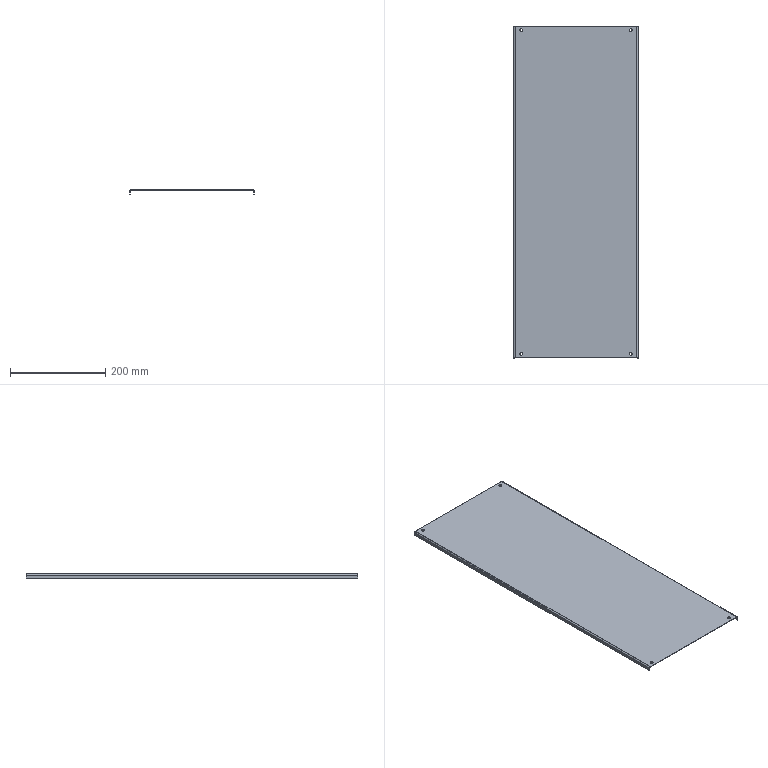Part | STEP file | Vertical arm guard plate (default) | 1 solid | 30 faces | box 262 x 698 x 9 mm | volume 192433 mm3 | plane 18 | cylinder 12 | commonest cylinder face diameters 6 x10 4 x2
STEP:
#1=CARTESIAN_POINT('',(-112.,340.,-1.));
#2=VERTEX_POINT('',#1);
#3=CARTESIAN_POINT('',(-118.,340.,-1.));
#4=VERTEX_POINT('',#3);
#5=CARTESIAN_POINT('',(-115.,340.,-1.));
#6=DIRECTION('',(0.,0.,-1.));
#7=DIRECTION('',(-1.,0.,0.));
#8=AXIS2_PLACEMENT_3D('',#5,#6,#7);
#9=CIRCLE('',#8,3.);
#10=EDGE_CURVE('',#2,#4,#9,.T.);
#11=ORIENTED_EDGE('',*,*,#10,.T.);
#12=CARTESIAN_POINT('',(-118.,340.,0.));
#13=VERTEX_POINT('',#12);
#14=CARTESIAN_POINT('',(-118.,340.,0.));
#15=DIRECTION('',(0.,0.,1.));
#16=VECTOR('',#15,1000.);
#17=LINE('',#14,#16);
#18=EDGE_CURVE('',#4,#13,#17,.T.);
#19=ORIENTED_EDGE('',*,*,#18,.T.);
#20=CARTESIAN_POINT('',(-112.,340.,0.));
#21=VERTEX_POINT('',#20);
#22=CARTESIAN_POINT('',(-115.,340.,0.));
#23=DIRECTION('',(0.,0.,1.));
#24=DIRECTION('',(1.,0.,0.));
#25=AXIS2_PLACEMENT_3D('',#22,#23,#24);
#26=CIRCLE('',#25,3.);
#27=EDGE_CURVE('',#13,#21,#26,.T.);
#28=ORIENTED_EDGE('',*,*,#27,.T.);
#29=CARTESIAN_POINT('',(-112.,340.,0.));
#30=DIRECTION('',(0.,0.,1.));
#31=VECTOR('',#30,1000.);
#32=LINE('',#29,#31);
#33=EDGE_CURVE('',#2,#21,#32,.T.);
#34=ORIENTED_EDGE('',*,*,#33,.F.);
#35=EDGE_LOOP('',(#11,#19,#28,#34));
#36=FACE_OUTER_BOUND('',#35,.T.);
#37=CARTESIAN_POINT('',(-115.,340.,0.));
#38=DIRECTION('',(0.,0.,1.));
#39=DIRECTION('',(1.,0.,0.));
#40=AXIS2_PLACEMENT_3D('',#37,#38,#39);
#41=CYLINDRICAL_SURFACE('',#40,3.);
#42=ADVANCED_FACE('',(#36),#41,.F.);
#43=CARTESIAN_POINT('',(118.,340.,-1.));
#44=VERTEX_POINT('',#43);
#45=CARTESIAN_POINT('',(112.,340.,-1.));
#46=VERTEX_POINT('',#45);
#47=CARTESIAN_POINT('',(115.,340.,-1.));
#48=DIRECTION('',(0.,0.,-1.));
#49=DIRECTION('',(-1.,0.,0.));
#50=AXIS2_PLACEMENT_3D('',#47,#48,#49);
#51=CIRCLE('',#50,3.);
#52=EDGE_CURVE('',#44,#46,#51,.T.);
#53=ORIENTED_EDGE('',*,*,#52,.T.);
#54=CARTESIAN_POINT('',(112.,340.,0.));
#55=VERTEX_POINT('',#54);
#56=CARTESIAN_POINT('',(112.,340.,0.));
#57=DIRECTION('',(0.,0.,1.));
#58=VECTOR('',#57,1000.);
#59=LINE('',#56,#58);
#60=EDGE_CURVE('',#46,#55,#59,.T.);
#61=ORIENTED_EDGE('',*,*,#60,.T.);
#62=CARTESIAN_POINT('',(118.,340.,0.));
#63=VERTEX_POINT('',#62);
#64=CARTESIAN_POINT('',(115.,340.,0.));
#65=DIRECTION('',(0.,0.,1.));
#66=DIRECTION('',(1.,0.,0.));
#67=AXIS2_PLACEMENT_3D('',#64,#65,#66);
#68=CIRCLE('',#67,3.);
#69=EDGE_CURVE('',#55,#63,#68,.T.);
#70=ORIENTED_EDGE('',*,*,#69,.T.);
#71=CARTESIAN_POINT('',(118.,340.,0.));
#72=DIRECTION('',(0.,0.,1.));
#73=VECTOR('',#72,1000.);
#74=LINE('',#71,#73);
#75=EDGE_CURVE('',#44,#63,#74,.T.);
#76=ORIENTED_EDGE('',*,*,#75,.F.);
#77=EDGE_LOOP('',(#53,#61,#70,#76));
#78=FACE_OUTER_BOUND('',#77,.T.);
#79=CARTESIAN_POINT('',(115.,340.,0.));
#80=DIRECTION('',(0.,0.,1.));
#81=DIRECTION('',(1.,0.,0.));
#82=AXIS2_PLACEMENT_3D('',#79,#80,#81);
#83=CYLINDRICAL_SURFACE('',#82,3.);
#84=ADVANCED_FACE('',(#78),#83,.F.);
#85=CARTESIAN_POINT('',(118.,-340.,-1.));
#86=VERTEX_POINT('',#85);
#87=CARTESIAN_POINT('',(112.,-340.,-1.));
#88=VERTEX_POINT('',#87);
#89=CARTESIAN_POINT('',(115.,-340.,-1.));
#90=DIRECTION('',(0.,0.,-1.));
#91=DIRECTION('',(-1.,0.,0.));
#92=AXIS2_PLACEMENT_3D('',#89,#90,#91);
#93=CIRCLE('',#92,3.);
#94=EDGE_CURVE('',#86,#88,#93,.T.);
#95=ORIENTED_EDGE('',*,*,#94,.T.);
#96=CARTESIAN_POINT('',(112.,-340.,0.));
#97=VERTEX_POINT('',#96);
#98=CARTESIAN_POINT('',(112.,-340.,0.));
#99=DIRECTION('',(0.,0.,1.));
#100=VECTOR('',#99,1000.);
#101=LINE('',#98,#100);
#102=EDGE_CURVE('',#88,#97,#101,.T.);
#103=ORIENTED_EDGE('',*,*,#102,.T.);
#104=CARTESIAN_POINT('',(118.,-340.,0.));
#105=VERTEX_POINT('',#104);
#106=CARTESIAN_POINT('',(115.,-340.,0.));
#107=DIRECTION('',(0.,0.,1.));
#108=DIRECTION('',(1.,0.,0.));
#109=AXIS2_PLACEMENT_3D('',#106,#107,#108);
#110=CIRCLE('',#109,3.);
#111=EDGE_CURVE('',#97,#105,#110,.T.);
#112=ORIENTED_EDGE('',*,*,#111,.T.);
#113=CARTESIAN_POINT('',(118.,-340.,0.));
#114=DIRECTION('',(0.,0.,1.));
#115=VECTOR('',#114,1000.);
#116=LINE('',#113,#115);
#117=EDGE_CURVE('',#86,#105,#116,.T.);
#118=ORIENTED_EDGE('',*,*,#117,.F.);
#119=EDGE_LOOP('',(#95,#103,#112,#118));
#120=FACE_OUTER_BOUND('',#119,.T.);
#121=CARTESIAN_POINT('',(115.,-340.,0.));
#122=DIRECTION('',(0.,0.,1.));
#123=DIRECTION('',(1.,0.,0.));
#124=AXIS2_PLACEMENT_3D('',#121,#122,#123);
#125=CYLINDRICAL_SURFACE('',#124,3.);
#126=ADVANCED_FACE('',(#120),#125,.F.);
#127=CARTESIAN_POINT('',(-112.,-340.,-1.));
#128=VERTEX_POINT('',#127);
#129=CARTESIAN_POINT('',(-118.,-340.,-1.));
#130=VERTEX_POINT('',#129);
#131=CARTESIAN_POINT('',(-115.,-340.,-1.));
#132=DIRECTION('',(0.,0.,-1.));
#133=DIRECTION('',(-1.,0.,0.));
#134=AXIS2_PLACEMENT_3D('',#131,#132,#133);
#135=CIRCLE('',#134,3.);
#136=EDGE_CURVE('',#128,#130,#135,.T.);
#137=ORIENTED_EDGE('',*,*,#136,.T.);
#138=CARTESIAN_POINT('',(-118.,-340.,0.));
#139=VERTEX_POINT('',#138);
#140=CARTESIAN_POINT('',(-118.,-340.,0.));
#141=DIRECTION('',(0.,0.,1.));
#142=VECTOR('',#141,1000.);
#143=LINE('',#140,#142);
#144=EDGE_CURVE('',#130,#139,#143,.T.);
#145=ORIENTED_EDGE('',*,*,#144,.T.);
#146=CARTESIAN_POINT('',(-112.,-340.,0.));
#147=VERTEX_POINT('',#146);
#148=CARTESIAN_POINT('',(-115.,-340.,0.));
#149=DIRECTION('',(0.,0.,1.));
#150=DIRECTION('',(1.,0.,0.));
#151=AXIS2_PLACEMENT_3D('',#148,#149,#150);
#152=CIRCLE('',#151,3.);
#153=EDGE_CURVE('',#139,#147,#152,.T.);
#154=ORIENTED_EDGE('',*,*,#153,.T.);
#155=CARTESIAN_POINT('',(-112.,-340.,0.));
#156=DIRECTION('',(0.,0.,1.));
#157=VECTOR('',#156,1000.);
#158=LINE('',#155,#157);
#159=EDGE_CURVE('',#128,#147,#158,.T.);
#160=ORIENTED_EDGE('',*,*,#159,.F.);
#161=EDGE_LOOP('',(#137,#145,#154,#160));
#162=FACE_OUTER_BOUND('',#161,.T.);
#163=CARTESIAN_POINT('',(-115.,-340.,0.));
#164=DIRECTION('',(0.,0.,1.));
#165=DIRECTION('',(1.,0.,0.));
#166=AXIS2_PLACEMENT_3D('',#163,#164,#165);
#167=CYLINDRICAL_SURFACE('',#166,3.);
#168=ADVANCED_FACE('',(#162),#167,.F.);
#169=ORIENTED_EDGE('',*,*,#10,.F.);
#170=CARTESIAN_POINT('',(-115.,340.,-1.));
#171=DIRECTION('',(0.,0.,-1.));
#172=DIRECTION('',(-1.,0.,0.));
#173=AXIS2_PLACEMENT_3D('',#170,#171,#172);
#174=CIRCLE('',#173,3.);
#175=EDGE_CURVE('',#4,#2,#174,.T.);
#176=ORIENTED_EDGE('',*,*,#175,.F.);
#177=EDGE_LOOP('',(#169,#176));
#178=FACE_BOUND('',#177,.T.);
#179=ORIENTED_EDGE('',*,*,#52,.F.);
#180=CARTESIAN_POINT('',(115.,340.,-1.));
#181=DIRECTION('',(0.,0.,-1.));
#182=DIRECTION('',(-1.,0.,0.));
#183=AXIS2_PLACEMENT_3D('',#180,#181,#182);
#184=CIRCLE('',#183,3.);
#185=EDGE_CURVE('',#46,#44,#184,.T.);
#186=ORIENTED_EDGE('',*,*,#185,.F.);
#187=EDGE_LOOP('',(#179,#186));
#188=FACE_BOUND('',#187,.T.);
#189=ORIENTED_EDGE('',*,*,#94,.F.);
#190=CARTESIAN_POINT('',(115.,-340.,-1.));
#191=DIRECTION('',(0.,0.,-1.));
#192=DIRECTION('',(-1.,0.,0.));
#193=AXIS2_PLACEMENT_3D('',#190,#191,#192);
#194=CIRCLE('',#193,3.);
#195=EDGE_CURVE('',#88,#86,#194,.T.);
#196=ORIENTED_EDGE('',*,*,#195,.F.);
#197=EDGE_LOOP('',(#189,#196));
#198=FACE_BOUND('',#197,.T.);
#199=ORIENTED_EDGE('',*,*,#136,.F.);
#200=CARTESIAN_POINT('',(-115.,-340.,-1.));
#201=DIRECTION('',(0.,0.,-1.));
#202=DIRECTION('',(-1.,0.,0.));
#203=AXIS2_PLACEMENT_3D('',#200,#201,#202);
#204=CIRCLE('',#203,3.);
#205=EDGE_CURVE('',#130,#128,#204,.T.);
#206=ORIENTED_EDGE('',*,*,#205,.F.);
#207=EDGE_LOOP('',(#199,#206));
#208=FACE_BOUND('',#207,.T.);
#209=CARTESIAN_POINT('',(-128.,-349.,-1.));
#210=VERTEX_POINT('',#209);
#211=CARTESIAN_POINT('',(128.,-349.,-1.));
#212=VERTEX_POINT('',#211);
#213=CARTESIAN_POINT('',(-130.,-349.,-1.));
#214=DIRECTION('',(1.,0.,0.));
#215=VECTOR('',#214,1000.);
#216=LINE('',#213,#215);
#217=EDGE_CURVE('',#210,#212,#216,.T.);
#218=ORIENTED_EDGE('',*,*,#217,.F.);
#219=CARTESIAN_POINT('',(-128.,349.,-1.));
#220=VERTEX_POINT('',#219);
#221=CARTESIAN_POINT('',(-128.,349.,-1.));
#222=DIRECTION('',(0.,-1.,0.));
#223=VECTOR('',#222,1000.);
#224=LINE('',#221,#223);
#225=EDGE_CURVE('',#220,#210,#224,.T.);
#226=ORIENTED_EDGE('',*,*,#225,.F.);
#227=CARTESIAN_POINT('',(128.,349.,-1.));
#228=VERTEX_POINT('',#227);
#229=CARTESIAN_POINT('',(-130.,349.,-1.));
#230=DIRECTION('',(-1.,0.,0.));
#231=VECTOR('',#230,1000.);
#232=LINE('',#229,#231);
#233=EDGE_CURVE('',#228,#220,#232,.T.);
#234=ORIENTED_EDGE('',*,*,#233,.F.);
#235=CARTESIAN_POINT('',(128.,-349.,-1.));
#236=DIRECTION('',(0.,1.,0.));
#237=VECTOR('',#236,1000.);
#238=LINE('',#235,#237);
#239=EDGE_CURVE('',#212,#228,#238,.T.);
#240=ORIENTED_EDGE('',*,*,#239,.F.);
#241=EDGE_LOOP('',(#218,#226,#234,#240));
#242=FACE_OUTER_BOUND('',#241,.T.);
#243=CARTESIAN_POINT('',(130.,349.,-1.));
#244=DIRECTION('',(0.,0.,-1.));
#245=DIRECTION('',(-1.,0.,0.));
#246=AXIS2_PLACEMENT_3D('',#243,#244,#245);
#247=PLANE('',#246);
#248=ADVANCED_FACE('',(#178,#188,#198,#208,#242),#247,.T.);
#249=CARTESIAN_POINT('',(-115.,340.,0.));
#250=DIRECTION('',(0.,0.,1.));
#251=DIRECTION('',(1.,0.,0.));
#252=AXIS2_PLACEMENT_3D('',#249,#250,#251);
#253=CIRCLE('',#252,3.);
#254=EDGE_CURVE('',#21,#13,#253,.T.);
#255=ORIENTED_EDGE('',*,*,#254,.F.);
#256=ORIENTED_EDGE('',*,*,#27,.F.);
#257=EDGE_LOOP('',(#255,#256));
#258=FACE_BOUND('',#257,.T.);
#259=CARTESIAN_POINT('',(115.,340.,0.));
#260=DIRECTION('',(0.,0.,1.));
#261=DIRECTION('',(1.,0.,0.));
#262=AXIS2_PLACEMENT_3D('',#259,#260,#261);
#263=CIRCLE('',#262,3.);
#264=EDGE_CURVE('',#63,#55,#263,.T.);
#265=ORIENTED_EDGE('',*,*,#264,.F.);
#266=ORIENTED_EDGE('',*,*,#69,.F.);
#267=EDGE_LOOP('',(#265,#266));
#268=FACE_BOUND('',#267,.T.);
#269=CARTESIAN_POINT('',(115.,-340.,0.));
#270=DIRECTION('',(0.,0.,1.));
#271=DIRECTION('',(1.,0.,0.));
#272=AXIS2_PLACEMENT_3D('',#269,#270,#271);
#273=CIRCLE('',#272,3.);
#274=EDGE_CURVE('',#105,#97,#273,.T.);
#275=ORIENTED_EDGE('',*,*,#274,.F.);
#276=ORIENTED_EDGE('',*,*,#111,.F.);
#277=EDGE_LOOP('',(#275,#276));
#278=FACE_BOUND('',#277,.T.);
#279=CARTESIAN_POINT('',(-115.,-340.,0.));
#280=DIRECTION('',(0.,0.,1.));
#281=DIRECTION('',(1.,0.,0.));
#282=AXIS2_PLACEMENT_3D('',#279,#280,#281);
#283=CIRCLE('',#282,3.);
#284=EDGE_CURVE('',#147,#139,#283,.T.);
#285=ORIENTED_EDGE('',*,*,#284,.F.);
#286=ORIENTED_EDGE('',*,*,#153,.F.);
#287=EDGE_LOOP('',(#285,#286));
#288=FACE_BOUND('',#287,.T.);
#289=CARTESIAN_POINT('',(-128.,349.,0.));
#290=VERTEX_POINT('',#289);
#291=CARTESIAN_POINT('',(-128.,-349.,0.));
#292=VERTEX_POINT('',#291);
#293=CARTESIAN_POINT('',(-128.,349.,0.));
#294=DIRECTION('',(0.,-1.,0.));
#295=VECTOR('',#294,1000.);
#296=LINE('',#293,#295);
#297=EDGE_CURVE('',#290,#292,#296,.T.);
#298=ORIENTED_EDGE('',*,*,#297,.T.);
#299=CARTESIAN_POINT('',(128.,-349.,0.));
#300=VERTEX_POINT('',#299);
#301=CARTESIAN_POINT('',(-130.,-349.,0.));
#302=DIRECTION('',(1.,0.,0.));
#303=VECTOR('',#302,1000.);
#304=LINE('',#301,#303);
#305=EDGE_CURVE('',#292,#300,#304,.T.);
#306=ORIENTED_EDGE('',*,*,#305,.T.);
#307=CARTESIAN_POINT('',(128.,349.,0.));
#308=VERTEX_POINT('',#307);
#309=CARTESIAN_POINT('',(128.,-349.,0.));
#310=DIRECTION('',(0.,1.,0.));
#311=VECTOR('',#310,1000.);
#312=LINE('',#309,#311);
#313=EDGE_CURVE('',#300,#308,#312,.T.);
#314=ORIENTED_EDGE('',*,*,#313,.T.);
#315=CARTESIAN_POINT('',(-130.,349.,0.));
#316=DIRECTION('',(-1.,0.,0.));
#317=VECTOR('',#316,1000.);
#318=LINE('',#315,#317);
#319=EDGE_CURVE('',#308,#290,#318,.T.);
#320=ORIENTED_EDGE('',*,*,#319,.T.);
#321=EDGE_LOOP('',(#298,#306,#314,#320));
#322=FACE_OUTER_BOUND('',#321,.T.);
#323=CARTESIAN_POINT('',(130.,349.,0.));
#324=DIRECTION('',(0.,0.,-1.));
#325=DIRECTION('',(-1.,0.,0.));
#326=AXIS2_PLACEMENT_3D('',#323,#324,#325);
#327=PLANE('',#326);
#328=ADVANCED_FACE('',(#258,#268,#278,#288,#322),#327,.F.);
#329=ORIENTED_EDGE('',*,*,#233,.T.);
#330=CARTESIAN_POINT('',(-128.,349.,-1.));
#331=DIRECTION('',(0.,0.,1.));
#332=VECTOR('',#331,1000.);
#333=LINE('',#330,#332);
#334=EDGE_CURVE('',#220,#290,#333,.T.);
#335=ORIENTED_EDGE('',*,*,#334,.T.);
#336=ORIENTED_EDGE('',*,*,#319,.F.);
#337=CARTESIAN_POINT('',(128.,349.,-1.));
#338=DIRECTION('',(0.,0.,1.));
#339=VECTOR('',#338,1000.);
#340=LINE('',#337,#339);
#341=EDGE_CURVE('',#228,#308,#340,.T.);
#342=ORIENTED_EDGE('',*,*,#341,.F.);
#343=EDGE_LOOP('',(#329,#335,#336,#342));
#344=FACE_OUTER_BOUND('',#343,.T.);
#345=CARTESIAN_POINT('',(-130.,349.,-1.));
#346=DIRECTION('',(0.,1.,0.));
#347=DIRECTION('',(0.,0.,1.));
#348=AXIS2_PLACEMENT_3D('',#345,#346,#347);
#349=PLANE('',#348);
#350=ADVANCED_FACE('',(#344),#349,.T.);
#351=CARTESIAN_POINT('',(-128.,-349.,-1.));
#352=DIRECTION('',(0.,0.,1.));
#353=VECTOR('',#352,1000.);
#354=LINE('',#351,#353);
#355=EDGE_CURVE('',#210,#292,#354,.T.);
#356=ORIENTED_EDGE('',*,*,#355,.F.);
#357=ORIENTED_EDGE('',*,*,#217,.T.);
#358=CARTESIAN_POINT('',(128.,-349.,-1.));
#359=DIRECTION('',(0.,0.,1.));
#360=VECTOR('',#359,1000.);
#361=LINE('',#358,#360);
#362=EDGE_CURVE('',#212,#300,#361,.T.);
#363=ORIENTED_EDGE('',*,*,#362,.T.);
#364=ORIENTED_EDGE('',*,*,#305,.F.);
#365=EDGE_LOOP('',(#356,#357,#363,#364));
#366=FACE_OUTER_BOUND('',#365,.T.);
#367=CARTESIAN_POINT('',(-130.,-349.,-1.));
#368=DIRECTION('',(0.,-1.,0.));
#369=DIRECTION('',(0.,0.,-1.));
#370=AXIS2_PLACEMENT_3D('',#367,#368,#369);
#371=PLANE('',#370);
#372=ADVANCED_FACE('',(#366),#371,.T.);
#373=ORIENTED_EDGE('',*,*,#144,.F.);
#374=ORIENTED_EDGE('',*,*,#205,.T.);
#375=ORIENTED_EDGE('',*,*,#159,.T.);
#376=ORIENTED_EDGE('',*,*,#284,.T.);
#377=EDGE_LOOP('',(#373,#374,#375,#376));
#378=FACE_OUTER_BOUND('',#377,.T.);
#379=CARTESIAN_POINT('',(-115.,-340.,0.));
#380=DIRECTION('',(0.,0.,1.));
#381=DIRECTION('',(1.,0.,0.));
#382=AXIS2_PLACEMENT_3D('',#379,#380,#381);
#383=CYLINDRICAL_SURFACE('',#382,3.);
#384=ADVANCED_FACE('',(#378),#383,.F.);
#385=ORIENTED_EDGE('',*,*,#102,.F.);
#386=ORIENTED_EDGE('',*,*,#195,.T.);
#387=ORIENTED_EDGE('',*,*,#117,.T.);
#388=ORIENTED_EDGE('',*,*,#274,.T.);
#389=EDGE_LOOP('',(#385,#386,#387,#388));
#390=FACE_OUTER_BOUND('',#389,.T.);
#391=CARTESIAN_POINT('',(115.,-340.,0.));
#392=DIRECTION('',(0.,0.,1.));
#393=DIRECTION('',(1.,0.,0.));
#394=AXIS2_PLACEMENT_3D('',#391,#392,#393);
#395=CYLINDRICAL_SURFACE('',#394,3.);
#396=ADVANCED_FACE('',(#390),#395,.F.);
#397=ORIENTED_EDGE('',*,*,#60,.F.);
#398=ORIENTED_EDGE('',*,*,#185,.T.);
#399=ORIENTED_EDGE('',*,*,#75,.T.);
#400=ORIENTED_EDGE('',*,*,#264,.T.);
#401=EDGE_LOOP('',(#397,#398,#399,#400));
#402=FACE_OUTER_BOUND('',#401,.T.);
#403=CARTESIAN_POINT('',(115.,340.,0.));
#404=DIRECTION('',(0.,0.,1.));
#405=DIRECTION('',(1.,0.,0.));
#406=AXIS2_PLACEMENT_3D('',#403,#404,#405);
#407=CYLINDRICAL_SURFACE('',#406,3.);
#408=ADVANCED_FACE('',(#402),#407,.F.);
#409=ORIENTED_EDGE('',*,*,#18,.F.);
#410=ORIENTED_EDGE('',*,*,#175,.T.);
#411=ORIENTED_EDGE('',*,*,#33,.T.);
#412=ORIENTED_EDGE('',*,*,#254,.T.);
#413=EDGE_LOOP('',(#409,#410,#411,#412));
#414=FACE_OUTER_BOUND('',#413,.T.);
#415=CARTESIAN_POINT('',(-115.,340.,0.));
#416=DIRECTION('',(0.,0.,1.));
#417=DIRECTION('',(1.,0.,0.));
#418=AXIS2_PLACEMENT_3D('',#415,#416,#417);
#419=CYLINDRICAL_SURFACE('',#418,3.);
#420=ADVANCED_FACE('',(#414),#419,.F.);
#421=CARTESIAN_POINT('',(130.,349.,-3.));
#422=VERTEX_POINT('',#421);
#423=CARTESIAN_POINT('',(131.,349.,-3.));
#424=VERTEX_POINT('',#423);
#425=CARTESIAN_POINT('',(130.,349.,-3.));
#426=DIRECTION('',(1.,0.,0.));
#427=VECTOR('',#426,1000.);
#428=LINE('',#425,#427);
#429=EDGE_CURVE('',#422,#424,#428,.T.);
#430=ORIENTED_EDGE('',*,*,#429,.F.);
#431=CARTESIAN_POINT('',(128.,349.,-3.));
#432=DIRECTION('',(0.,1.,0.));
#433=DIRECTION('',(0.,0.,-1.));
#434=AXIS2_PLACEMENT_3D('',#431,#432,#433);
#435=CIRCLE('',#434,2.);
#436=EDGE_CURVE('',#228,#422,#435,.T.);
#437=ORIENTED_EDGE('',*,*,#436,.F.);
#438=ORIENTED_EDGE('',*,*,#341,.T.);
#439=CARTESIAN_POINT('',(128.,349.,-3.));
#440=DIRECTION('',(0.,1.,0.));
#441=DIRECTION('',(0.,0.,-1.));
#442=AXIS2_PLACEMENT_3D('',#439,#440,#441);
#443=CIRCLE('',#442,3.);
#444=EDGE_CURVE('',#308,#424,#443,.T.);
#445=ORIENTED_EDGE('',*,*,#444,.T.);
#446=EDGE_LOOP('',(#430,#437,#438,#445));
#447=FACE_OUTER_BOUND('',#446,.T.);
#448=CARTESIAN_POINT('',(128.,349.,-3.));
#449=DIRECTION('',(0.,1.,0.));
#450=DIRECTION('',(0.,0.,1.));
#451=AXIS2_PLACEMENT_3D('',#448,#449,#450);
#452=PLANE('',#451);
#453=ADVANCED_FACE('',(#447),#452,.T.);
#454=CARTESIAN_POINT('',(130.,-349.,-3.));
#455=VERTEX_POINT('',#454);
#456=CARTESIAN_POINT('',(128.,-349.,-3.));
#457=DIRECTION('',(0.,-1.,0.));
#458=DIRECTION('',(0.,0.,-1.));
#459=AXIS2_PLACEMENT_3D('',#456,#457,#458);
#460=CIRCLE('',#459,2.);
#461=EDGE_CURVE('',#455,#212,#460,.T.);
#462=ORIENTED_EDGE('',*,*,#461,.F.);
#463=CARTESIAN_POINT('',(131.,-349.,-3.));
#464=VERTEX_POINT('',#463);
#465=CARTESIAN_POINT('',(130.,-349.,-3.));
#466=DIRECTION('',(1.,0.,0.));
#467=VECTOR('',#466,1000.);
#468=LINE('',#465,#467);
#469=EDGE_CURVE('',#455,#464,#468,.T.);
#470=ORIENTED_EDGE('',*,*,#469,.T.);
#471=CARTESIAN_POINT('',(128.,-349.,-3.));
#472=DIRECTION('',(0.,-1.,0.));
#473=DIRECTION('',(0.,0.,-1.));
#474=AXIS2_PLACEMENT_3D('',#471,#472,#473);
#475=CIRCLE('',#474,3.);
#476=EDGE_CURVE('',#464,#300,#475,.T.);
#477=ORIENTED_EDGE('',*,*,#476,.T.);
#478=ORIENTED_EDGE('',*,*,#362,.F.);
#479=EDGE_LOOP('',(#462,#470,#477,#478));
#480=FACE_OUTER_BOUND('',#479,.T.);
#481=CARTESIAN_POINT('',(128.,-349.,-3.));
#482=DIRECTION('',(0.,1.,0.));
#483=DIRECTION('',(0.,0.,1.));
#484=AXIS2_PLACEMENT_3D('',#481,#482,#483);
#485=PLANE('',#484);
#486=ADVANCED_FACE('',(#480),#485,.F.);
#487=ORIENTED_EDGE('',*,*,#313,.F.);
#488=ORIENTED_EDGE('',*,*,#476,.F.);
#489=CARTESIAN_POINT('',(131.,-349.,-3.));
#490=DIRECTION('',(0.,-1.,0.));
#491=VECTOR('',#490,1000.);
#492=LINE('',#489,#491);
#493=EDGE_CURVE('',#424,#464,#492,.T.);
#494=ORIENTED_EDGE('',*,*,#493,.F.);
#495=ORIENTED_EDGE('',*,*,#444,.F.);
#496=EDGE_LOOP('',(#487,#488,#494,#495));
#497=FACE_OUTER_BOUND('',#496,.T.);
#498=CARTESIAN_POINT('',(128.,-349.,-3.));
#499=DIRECTION('',(0.,-1.,0.));
#500=DIRECTION('',(1.,0.,0.));
#501=AXIS2_PLACEMENT_3D('',#498,#499,#500);
#502=CYLINDRICAL_SURFACE('',#501,3.);
#503=ADVANCED_FACE('',(#497),#502,.T.);
#504=ORIENTED_EDGE('',*,*,#239,.T.);
#505=ORIENTED_EDGE('',*,*,#436,.T.);
#506=CARTESIAN_POINT('',(130.,349.,-3.));
#507=DIRECTION('',(0.,-1.,0.));
#508=VECTOR('',#507,1000.);
#509=LINE('',#506,#508);
#510=EDGE_CURVE('',#422,#455,#509,.T.);
#511=ORIENTED_EDGE('',*,*,#510,.T.);
#512=ORIENTED_EDGE('',*,*,#461,.T.);
#513=EDGE_LOOP('',(#504,#505,#511,#512));
#514=FACE_OUTER_BOUND('',#513,.T.);
#515=CARTESIAN_POINT('',(128.,-349.,-3.));
#516=DIRECTION('',(0.,-1.,0.));
#517=DIRECTION('',(1.,0.,0.));
#518=AXIS2_PLACEMENT_3D('',#515,#516,#517);
#519=CYLINDRICAL_SURFACE('',#518,2.);
#520=ADVANCED_FACE('',(#514),#519,.F.);
#521=CARTESIAN_POINT('',(131.,-349.,-9.));
#522=VERTEX_POINT('',#521);
#523=CARTESIAN_POINT('',(131.,-349.,-1.));
#524=DIRECTION('',(0.,0.,1.));
#525=VECTOR('',#524,1000.);
#526=LINE('',#523,#525);
#527=EDGE_CURVE('',#522,#464,#526,.T.);
#528=ORIENTED_EDGE('',*,*,#527,.T.);
#529=ORIENTED_EDGE('',*,*,#469,.F.);
#530=CARTESIAN_POINT('',(130.,-349.,-9.));
#531=VERTEX_POINT('',#530);
#532=CARTESIAN_POINT('',(130.,-349.,-1.));
#533=DIRECTION('',(0.,0.,1.));
#534=VECTOR('',#533,1000.);
#535=LINE('',#532,#534);
#536=EDGE_CURVE('',#531,#455,#535,.T.);
#537=ORIENTED_EDGE('',*,*,#536,.F.);
#538=CARTESIAN_POINT('',(131.,-349.,-9.));
#539=DIRECTION('',(-1.,0.,0.));
#540=VECTOR('',#539,1000.);
#541=LINE('',#538,#540);
#542=EDGE_CURVE('',#522,#531,#541,.T.);
#543=ORIENTED_EDGE('',*,*,#542,.F.);
#544=EDGE_LOOP('',(#528,#529,#537,#543));
#545=FACE_OUTER_BOUND('',#544,.T.);
#546=CARTESIAN_POINT('',(131.,-349.,-1.));
#547=DIRECTION('',(0.,-1.,0.));
#548=DIRECTION('',(0.,0.,-1.));
#549=AXIS2_PLACEMENT_3D('',#546,#547,#548);
#550=PLANE('',#549);
#551=ADVANCED_FACE('',(#545),#550,.T.);
#552=CARTESIAN_POINT('',(130.,349.,-9.));
#553=VERTEX_POINT('',#552);
#554=CARTESIAN_POINT('',(130.,349.,-9.));
#555=DIRECTION('',(0.,0.,-1.));
#556=VECTOR('',#555,1000.);
#557=LINE('',#554,#556);
#558=EDGE_CURVE('',#422,#553,#557,.T.);
#559=ORIENTED_EDGE('',*,*,#558,.F.);
#560=ORIENTED_EDGE('',*,*,#429,.T.);
#561=CARTESIAN_POINT('',(131.,349.,-9.));
#562=VERTEX_POINT('',#561);
#563=CARTESIAN_POINT('',(131.,349.,-9.));
#564=DIRECTION('',(0.,0.,-1.));
#565=VECTOR('',#564,1000.);
#566=LINE('',#563,#565);
#567=EDGE_CURVE('',#424,#562,#566,.T.);
#568=ORIENTED_EDGE('',*,*,#567,.T.);
#569=CARTESIAN_POINT('',(131.,349.,-9.));
#570=DIRECTION('',(-1.,0.,0.));
#571=VECTOR('',#570,1000.);
#572=LINE('',#569,#571);
#573=EDGE_CURVE('',#562,#553,#572,.T.);
#574=ORIENTED_EDGE('',*,*,#573,.T.);
#575=EDGE_LOOP('',(#559,#560,#568,#574));
#576=FACE_OUTER_BOUND('',#575,.T.);
#577=CARTESIAN_POINT('',(131.,349.,-9.));
#578=DIRECTION('',(0.,1.,0.));
#579=DIRECTION('',(0.,0.,1.));
#580=AXIS2_PLACEMENT_3D('',#577,#578,#579);
#581=PLANE('',#580);
#582=ADVANCED_FACE('',(#576),#581,.T.);
#583=ORIENTED_EDGE('',*,*,#567,.F.);
#584=ORIENTED_EDGE('',*,*,#493,.T.);
#585=ORIENTED_EDGE('',*,*,#527,.F.);
#586=CARTESIAN_POINT('',(131.,-349.,-9.));
#587=DIRECTION('',(0.,-1.,0.));
#588=VECTOR('',#587,1000.);
#589=LINE('',#586,#588);
#590=EDGE_CURVE('',#562,#522,#589,.T.);
#591=ORIENTED_EDGE('',*,*,#590,.F.);
#592=EDGE_LOOP('',(#583,#584,#585,#591));
#593=FACE_OUTER_BOUND('',#592,.T.);
#594=CARTESIAN_POINT('',(131.,-349.,-1.));
#595=DIRECTION('',(1.,0.,0.));
#596=DIRECTION('',(0.,0.,-1.));
#597=AXIS2_PLACEMENT_3D('',#594,#595,#596);
#598=PLANE('',#597);
#599=ADVANCED_FACE('',(#593),#598,.T.);
#600=ORIENTED_EDGE('',*,*,#510,.F.);
#601=ORIENTED_EDGE('',*,*,#558,.T.);
#602=CARTESIAN_POINT('',(130.,-349.,-9.));
#603=DIRECTION('',(0.,-1.,0.));
#604=VECTOR('',#603,1000.);
#605=LINE('',#602,#604);
#606=EDGE_CURVE('',#553,#531,#605,.T.);
#607=ORIENTED_EDGE('',*,*,#606,.T.);
#608=ORIENTED_EDGE('',*,*,#536,.T.);
#609=EDGE_LOOP('',(#600,#601,#607,#608));
#610=FACE_OUTER_BOUND('',#609,.T.);
#611=CARTESIAN_POINT('',(130.,-349.,-1.));
#612=DIRECTION('',(1.,0.,0.));
#613=DIRECTION('',(0.,0.,-1.));
#614=AXIS2_PLACEMENT_3D('',#611,#612,#613);
#615=PLANE('',#614);
#616=ADVANCED_FACE('',(#610),#615,.F.);
#617=ORIENTED_EDGE('',*,*,#606,.F.);
#618=ORIENTED_EDGE('',*,*,#573,.F.);
#619=ORIENTED_EDGE('',*,*,#590,.T.);
#620=ORIENTED_EDGE('',*,*,#542,.T.);
#621=EDGE_LOOP('',(#617,#618,#619,#620));
#622=FACE_OUTER_BOUND('',#621,.T.);
#623=CARTESIAN_POINT('',(131.,-349.,-9.));
#624=DIRECTION('',(0.,0.,-1.));
#625=DIRECTION('',(-1.,0.,0.));
#626=AXIS2_PLACEMENT_3D('',#623,#624,#625);
#627=PLANE('',#626);
#628=ADVANCED_FACE('',(#622),#627,.T.);
#629=CARTESIAN_POINT('',(-130.,-349.,-3.));
#630=VERTEX_POINT('',#629);
#631=CARTESIAN_POINT('',(-131.,-349.,-3.));
#632=VERTEX_POINT('',#631);
#633=CARTESIAN_POINT('',(-130.,-349.,-3.));
#634=DIRECTION('',(-1.,0.,0.));
#635=VECTOR('',#634,1000.);
#636=LINE('',#633,#635);
#637=EDGE_CURVE('',#630,#632,#636,.T.);
#638=ORIENTED_EDGE('',*,*,#637,.F.);
#639=CARTESIAN_POINT('',(-128.,-349.,-3.));
#640=DIRECTION('',(0.,-1.,0.));
#641=DIRECTION('',(0.,0.,1.));
#642=AXIS2_PLACEMENT_3D('',#639,#640,#641);
#643=CIRCLE('',#642,2.);
#644=EDGE_CURVE('',#210,#630,#643,.T.);
#645=ORIENTED_EDGE('',*,*,#644,.F.);
#646=ORIENTED_EDGE('',*,*,#355,.T.);
#647=CARTESIAN_POINT('',(-128.,-349.,-3.));
#648=DIRECTION('',(0.,-1.,0.));
#649=DIRECTION('',(0.,0.,1.));
#650=AXIS2_PLACEMENT_3D('',#647,#648,#649);
#651=CIRCLE('',#650,3.);
#652=EDGE_CURVE('',#292,#632,#651,.T.);
#653=ORIENTED_EDGE('',*,*,#652,.T.);
#654=EDGE_LOOP('',(#638,#645,#646,#653));
#655=FACE_OUTER_BOUND('',#654,.T.);
#656=CARTESIAN_POINT('',(-128.,-349.,-3.));
#657=DIRECTION('',(0.,-1.,0.));
#658=DIRECTION('',(0.,0.,-1.));
#659=AXIS2_PLACEMENT_3D('',#656,#657,#658);
#660=PLANE('',#659);
#661=ADVANCED_FACE('',(#655),#660,.T.);
#662=CARTESIAN_POINT('',(-130.,349.,-3.));
#663=VERTEX_POINT('',#662);
#664=CARTESIAN_POINT('',(-128.,349.,-3.));
#665=DIRECTION('',(0.,1.,0.));
#666=DIRECTION('',(0.,0.,1.));
#667=AXIS2_PLACEMENT_3D('',#664,#665,#666);
#668=CIRCLE('',#667,2.);
#669=EDGE_CURVE('',#663,#220,#668,.T.);
#670=ORIENTED_EDGE('',*,*,#669,.F.);
#671=CARTESIAN_POINT('',(-131.,349.,-3.));
#672=VERTEX_POINT('',#671);
#673=CARTESIAN_POINT('',(-130.,349.,-3.));
#674=DIRECTION('',(-1.,0.,0.));
#675=VECTOR('',#674,1000.);
#676=LINE('',#673,#675);
#677=EDGE_CURVE('',#663,#672,#676,.T.);
#678=ORIENTED_EDGE('',*,*,#677,.T.);
#679=CARTESIAN_POINT('',(-128.,349.,-3.));
#680=DIRECTION('',(0.,1.,0.));
#681=DIRECTION('',(0.,0.,1.));
#682=AXIS2_PLACEMENT_3D('',#679,#680,#681);
#683=CIRCLE('',#682,3.);
#684=EDGE_CURVE('',#672,#290,#683,.T.);
#685=ORIENTED_EDGE('',*,*,#684,.T.);
#686=ORIENTED_EDGE('',*,*,#334,.F.);
#687=EDGE_LOOP('',(#670,#678,#685,#686));
#688=FACE_OUTER_BOUND('',#687,.T.);
#689=CARTESIAN_POINT('',(-128.,349.,-3.));
#690=DIRECTION('',(0.,-1.,0.));
#691=DIRECTION('',(0.,0.,-1.));
#692=AXIS2_PLACEMENT_3D('',#689,#690,#691);
#693=PLANE('',#692);
#694=ADVANCED_FACE('',(#688),#693,.F.);
#695=ORIENTED_EDGE('',*,*,#297,.F.);
#696=ORIENTED_EDGE('',*,*,#684,.F.);
#697=CARTESIAN_POINT('',(-131.,-349.,-3.));
#698=DIRECTION('',(0.,-1.,0.));
#699=VECTOR('',#698,1000.);
#700=LINE('',#697,#699);
#701=EDGE_CURVE('',#672,#632,#700,.T.);
#702=ORIENTED_EDGE('',*,*,#701,.T.);
#703=ORIENTED_EDGE('',*,*,#652,.F.);
#704=EDGE_LOOP('',(#695,#696,#702,#703));
#705=FACE_OUTER_BOUND('',#704,.T.);
#706=CARTESIAN_POINT('',(-128.,349.,-3.));
#707=DIRECTION('',(0.,1.,0.));
#708=DIRECTION('',(-1.,0.,0.));
#709=AXIS2_PLACEMENT_3D('',#706,#707,#708);
#710=CYLINDRICAL_SURFACE('',#709,3.);
#711=ADVANCED_FACE('',(#705),#710,.T.);
#712=ORIENTED_EDGE('',*,*,#225,.T.);
#713=ORIENTED_EDGE('',*,*,#644,.T.);
#714=CARTESIAN_POINT('',(-130.,-349.,-3.));
#715=DIRECTION('',(0.,1.,0.));
#716=VECTOR('',#715,1000.);
#717=LINE('',#714,#716);
#718=EDGE_CURVE('',#630,#663,#717,.T.);
#719=ORIENTED_EDGE('',*,*,#718,.T.);
#720=ORIENTED_EDGE('',*,*,#669,.T.);
#721=EDGE_LOOP('',(#712,#713,#719,#720));
#722=FACE_OUTER_BOUND('',#721,.T.);
#723=CARTESIAN_POINT('',(-128.,349.,-3.));
#724=DIRECTION('',(0.,1.,0.));
#725=DIRECTION('',(-1.,0.,0.));
#726=AXIS2_PLACEMENT_3D('',#723,#724,#725);
#727=CYLINDRICAL_SURFACE('',#726,2.);
#728=ADVANCED_FACE('',(#722),#727,.F.);
#729=CARTESIAN_POINT('',(-130.,-349.,-9.));
#730=VERTEX_POINT('',#729);
#731=CARTESIAN_POINT('',(-130.,-349.,-1.));
#732=DIRECTION('',(0.,0.,-1.));
#733=VECTOR('',#732,1000.);
#734=LINE('',#731,#733);
#735=EDGE_CURVE('',#630,#730,#734,.T.);
#736=ORIENTED_EDGE('',*,*,#735,.F.);
#737=ORIENTED_EDGE('',*,*,#637,.T.);
#738=CARTESIAN_POINT('',(-131.,-349.,-9.));
#739=VERTEX_POINT('',#738);
#740=CARTESIAN_POINT('',(-131.,-349.,-1.));
#741=DIRECTION('',(0.,0.,-1.));
#742=VECTOR('',#741,1000.);
#743=LINE('',#740,#742);
#744=EDGE_CURVE('',#632,#739,#743,.T.);
#745=ORIENTED_EDGE('',*,*,#744,.T.);
#746=CARTESIAN_POINT('',(-131.,-349.,-9.));
#747=DIRECTION('',(1.,0.,0.));
#748=VECTOR('',#747,1000.);
#749=LINE('',#746,#748);
#750=EDGE_CURVE('',#739,#730,#749,.T.);
#751=ORIENTED_EDGE('',*,*,#750,.T.);
#752=EDGE_LOOP('',(#736,#737,#745,#751));
#753=FACE_OUTER_BOUND('',#752,.T.);
#754=CARTESIAN_POINT('',(-131.,-349.,-1.));
#755=DIRECTION('',(0.,-1.,0.));
#756=DIRECTION('',(0.,0.,-1.));
#757=AXIS2_PLACEMENT_3D('',#754,#755,#756);
#758=PLANE('',#757);
#759=ADVANCED_FACE('',(#753),#758,.T.);
#760=CARTESIAN_POINT('',(-131.,349.,-9.));
#761=VERTEX_POINT('',#760);
#762=CARTESIAN_POINT('',(-131.,349.,-9.));
#763=DIRECTION('',(0.,0.,1.));
#764=VECTOR('',#763,1000.);
#765=LINE('',#762,#764);
#766=EDGE_CURVE('',#761,#672,#765,.T.);
#767=ORIENTED_EDGE('',*,*,#766,.T.);
#768=ORIENTED_EDGE('',*,*,#677,.F.);
#769=CARTESIAN_POINT('',(-130.,349.,-9.));
#770=VERTEX_POINT('',#769);
#771=CARTESIAN_POINT('',(-130.,349.,-9.));
#772=DIRECTION('',(0.,0.,1.));
#773=VECTOR('',#772,1000.);
#774=LINE('',#771,#773);
#775=EDGE_CURVE('',#770,#663,#774,.T.);
#776=ORIENTED_EDGE('',*,*,#775,.F.);
#777=CARTESIAN_POINT('',(-131.,349.,-9.));
#778=DIRECTION('',(1.,0.,0.));
#779=VECTOR('',#778,1000.);
#780=LINE('',#777,#779);
#781=EDGE_CURVE('',#761,#770,#780,.T.);
#782=ORIENTED_EDGE('',*,*,#781,.F.);
#783=EDGE_LOOP('',(#767,#768,#776,#782));
#784=FACE_OUTER_BOUND('',#783,.T.);
#785=CARTESIAN_POINT('',(-131.,349.,-9.));
#786=DIRECTION('',(0.,1.,0.));
#787=DIRECTION('',(0.,0.,1.));
#788=AXIS2_PLACEMENT_3D('',#785,#786,#787);
#789=PLANE('',#788);
#790=ADVANCED_FACE('',(#784),#789,.T.);
#791=ORIENTED_EDGE('',*,*,#701,.F.);
#792=ORIENTED_EDGE('',*,*,#766,.F.);
#793=CARTESIAN_POINT('',(-131.,-349.,-9.));
#794=DIRECTION('',(0.,1.,0.));
#795=VECTOR('',#794,1000.);
#796=LINE('',#793,#795);
#797=EDGE_CURVE('',#739,#761,#796,.T.);
#798=ORIENTED_EDGE('',*,*,#797,.F.);
#799=ORIENTED_EDGE('',*,*,#744,.F.);
#800=EDGE_LOOP('',(#791,#792,#798,#799));
#801=FACE_OUTER_BOUND('',#800,.T.);
#802=CARTESIAN_POINT('',(-131.,-349.,-9.));
#803=DIRECTION('',(1.,0.,0.));
#804=DIRECTION('',(0.,0.,-1.));
#805=AXIS2_PLACEMENT_3D('',#802,#803,#804);
#806=PLANE('',#805);
#807=ADVANCED_FACE('',(#801),#806,.F.);
#808=ORIENTED_EDGE('',*,*,#775,.T.);
#809=ORIENTED_EDGE('',*,*,#718,.F.);
#810=ORIENTED_EDGE('',*,*,#735,.T.);
#811=CARTESIAN_POINT('',(-130.,-349.,-9.));
#812=DIRECTION('',(0.,1.,0.));
#813=VECTOR('',#812,1000.);
#814=LINE('',#811,#813);
#815=EDGE_CURVE('',#730,#770,#814,.T.);
#816=ORIENTED_EDGE('',*,*,#815,.T.);
#817=EDGE_LOOP('',(#808,#809,#810,#816));
#818=FACE_OUTER_BOUND('',#817,.T.);
#819=CARTESIAN_POINT('',(-130.,-349.,-9.));
#820=DIRECTION('',(1.,0.,0.));
#821=DIRECTION('',(0.,0.,-1.));
#822=AXIS2_PLACEMENT_3D('',#819,#820,#821);
#823=PLANE('',#822);
#824=ADVANCED_FACE('',(#818),#823,.T.);
#825=ORIENTED_EDGE('',*,*,#815,.F.);
#826=ORIENTED_EDGE('',*,*,#750,.F.);
#827=ORIENTED_EDGE('',*,*,#797,.T.);
#828=ORIENTED_EDGE('',*,*,#781,.T.);
#829=EDGE_LOOP('',(#825,#826,#827,#828));
#830=FACE_OUTER_BOUND('',#829,.T.);
#831=CARTESIAN_POINT('',(-131.,-349.,-9.));
#832=DIRECTION('',(0.,0.,-1.));
#833=DIRECTION('',(-1.,0.,0.));
#834=AXIS2_PLACEMENT_3D('',#831,#832,#833);
#835=PLANE('',#834);
#836=ADVANCED_FACE('',(#830),#835,.T.);
#837=CLOSED_SHELL('',(#42,#84,#126,#168,#248,#328,#350,#372,#384,#396,#408,#420,#453,#486,#503,#520,#551,#582,#599,#616,#628,#661,#694,#711,#728,#759,#790,#807,#824,#836));
#838=MANIFOLD_SOLID_BREP('',#837);
#839=CARTESIAN_POINT('',(0.,0.,0.));
#840=DIRECTION('',(0.,0.,1.));
#841=DIRECTION('',(1.,0.,0.));
#842=AXIS2_PLACEMENT_3D('',#839,#840,#841);
#843=(LENGTH_UNIT()NAMED_UNIT(*)SI_UNIT(.MILLI.,.METRE.));
#844=UNCERTAINTY_MEASURE_WITH_UNIT(LENGTH_MEASURE(0.00001),#843,'','');
#845=(NAMED_UNIT(*)PLANE_ANGLE_UNIT()SI_UNIT($,.RADIAN.));
#846=(NAMED_UNIT(*)SI_UNIT($,.STERADIAN.)SOLID_ANGLE_UNIT());
#847=(GEOMETRIC_REPRESENTATION_CONTEXT(3)GLOBAL_UNCERTAINTY_ASSIGNED_CONTEXT((#844))GLOBAL_UNIT_ASSIGNED_CONTEXT((#843,#845,#846))REPRESENTATION_CONTEXT('',''));
#848=ADVANCED_BREP_SHAPE_REPRESENTATION('',(#838,#842),#847);